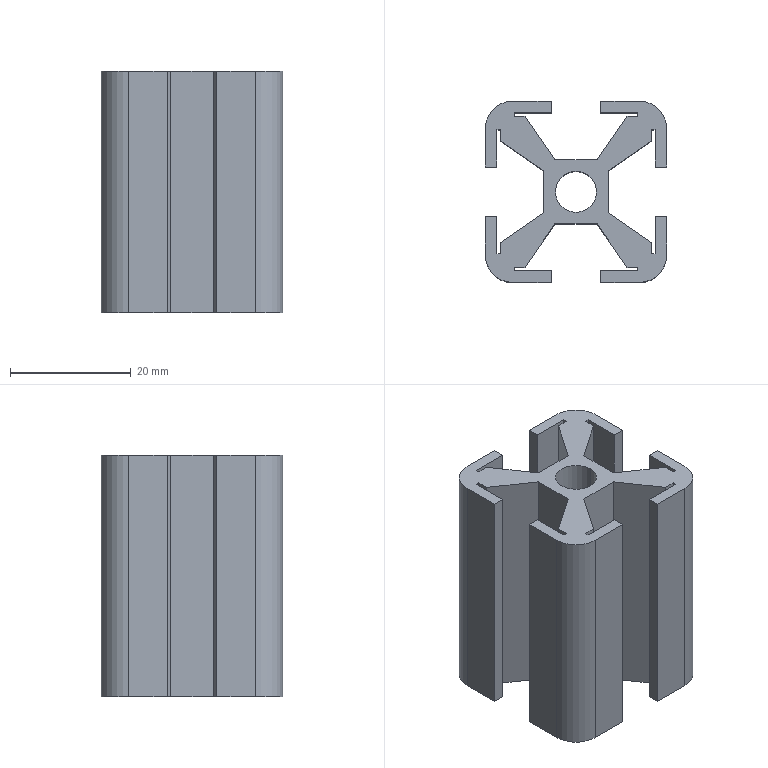Part | SolidWorks | features CirPattern 1, Extrusion 1, Fillet 1, ICE 1 | 1 solid | 60 faces | box 30 x 30 x 40 mm | volume 15672 mm3 | plane 54 | cylinder 6 | commonest cylinder face diameters 9 x4 6.8 x2